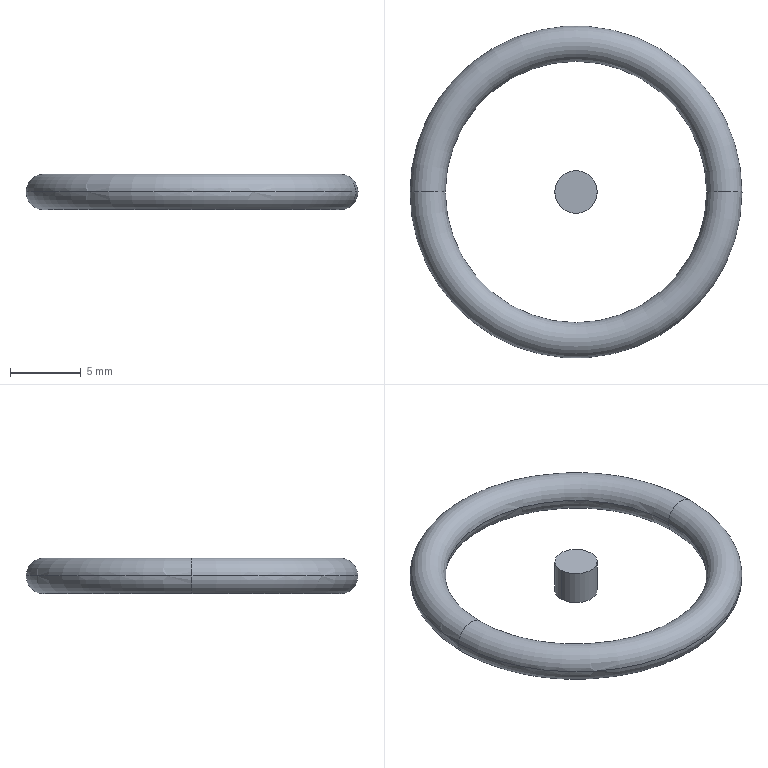Part | STEP file | O-ring 11 diameter after expansion 19 | 2 solids | 8 faces | box 23.5 x 23.5 x 2.5 mm | volume 341.518 mm3 | torus 4 | cylinder 2 | plane 2 | commonest cylinder face diameters 3 x2
STEP:
#1=CARTESIAN_POINT('',(0.,0.,0.));
#2=DIRECTION('',(0.,0.,1.));
#3=DIRECTION('',(1.,0.,0.));
#4=AXIS2_PLACEMENT_3D('',#1,#2,#3);
#5=CARTESIAN_POINT('',(-11.75,0.,0.));
#6=VERTEX_POINT('',#5);
#7=CARTESIAN_POINT('',(-9.25,0.,0.));
#8=VERTEX_POINT('',#7);
#9=CARTESIAN_POINT('',(-10.5,0.,0.));
#10=DIRECTION('',(0.,1.,0.));
#11=DIRECTION('',(-1.,0.,0.));
#12=AXIS2_PLACEMENT_3D('',#9,#10,#11);
#13=CIRCLE('',#12,1.25);
#14=CARTESIAN_POINT('',(0.,0.,0.));
#15=DIRECTION('',(0.,0.,1.));
#16=DIRECTION('',(1.,0.,0.));
#17=AXIS2_PLACEMENT_3D('',#14,#15,#16);
#18=TOROIDAL_SURFACE('',#17,10.5,1.25);
#19=CARTESIAN_POINT('',(3.142,0.));
#20=DIRECTION('',(0.,1.));
#21=VECTOR('',#20,1.);
#22=LINE('',#19,#21);
#23=(GEOMETRIC_REPRESENTATION_CONTEXT(2)PARAMETRIC_REPRESENTATION_CONTEXT()REPRESENTATION_CONTEXT('',''));
#24=DEFINITIONAL_REPRESENTATION('',(#22),#23);
#25=PCURVE('',#18,#24);
#26=CARTESIAN_POINT('',(0.,0.,0.));
#27=DIRECTION('',(0.,0.,1.));
#28=DIRECTION('',(1.,0.,0.));
#29=AXIS2_PLACEMENT_3D('',#26,#27,#28);
#30=TOROIDAL_SURFACE('',#29,10.5,1.25);
#31=CARTESIAN_POINT('',(3.142,0.));
#32=DIRECTION('',(0.,1.));
#33=VECTOR('',#32,1.);
#34=LINE('',#31,#33);
#35=(GEOMETRIC_REPRESENTATION_CONTEXT(2)PARAMETRIC_REPRESENTATION_CONTEXT()REPRESENTATION_CONTEXT('',''));
#36=DEFINITIONAL_REPRESENTATION('',(#34),#35);
#37=PCURVE('',#30,#36);
#38=SURFACE_CURVE('',#13,(#25,#37),.PCURVE_S1.);
#39=EDGE_CURVE('',#6,#8,#38,.T.);
#40=ORIENTED_EDGE('',*,*,#39,.F.);
#41=CARTESIAN_POINT('',(11.75,0.,0.));
#42=VERTEX_POINT('',#41);
#43=CARTESIAN_POINT('',(0.,0.,0.));
#44=DIRECTION('',(0.,0.,1.));
#45=DIRECTION('',(1.,0.,0.));
#46=AXIS2_PLACEMENT_3D('',#43,#44,#45);
#47=CIRCLE('',#46,11.75);
#48=CARTESIAN_POINT('',(0.,0.));
#49=DIRECTION('',(1.,0.));
#50=VECTOR('',#49,1.);
#51=LINE('',#48,#50);
#52=(GEOMETRIC_REPRESENTATION_CONTEXT(2)PARAMETRIC_REPRESENTATION_CONTEXT()REPRESENTATION_CONTEXT('',''));
#53=DEFINITIONAL_REPRESENTATION('',(#51),#52);
#54=PCURVE('',#18,#53);
#55=CARTESIAN_POINT('',(0.,0.,0.));
#56=DIRECTION('',(0.,0.,1.));
#57=DIRECTION('',(1.,0.,0.));
#58=AXIS2_PLACEMENT_3D('',#55,#56,#57);
#59=TOROIDAL_SURFACE('',#58,10.5,1.25);
#60=CARTESIAN_POINT('',(0.,6.283));
#61=DIRECTION('',(1.,0.));
#62=VECTOR('',#61,1.);
#63=LINE('',#60,#62);
#64=(GEOMETRIC_REPRESENTATION_CONTEXT(2)PARAMETRIC_REPRESENTATION_CONTEXT()REPRESENTATION_CONTEXT('',''));
#65=DEFINITIONAL_REPRESENTATION('',(#63),#64);
#66=PCURVE('',#59,#65);
#67=SURFACE_CURVE('',#47,(#54,#66),.PCURVE_S1.);
#68=EDGE_CURVE('',#6,#42,#67,.T.);
#69=ORIENTED_EDGE('',*,*,#68,.T.);
#70=CARTESIAN_POINT('',(9.25,0.,0.));
#71=VERTEX_POINT('',#70);
#72=CARTESIAN_POINT('',(10.5,0.,0.));
#73=DIRECTION('',(0.,-1.,0.));
#74=DIRECTION('',(0.,0.,-1.));
#75=AXIS2_PLACEMENT_3D('',#72,#73,#74);
#76=CIRCLE('',#75,1.25);
#77=CARTESIAN_POINT('',(6.283,-1.571));
#78=DIRECTION('',(0.,1.));
#79=VECTOR('',#78,1.);
#80=LINE('',#77,#79);
#81=(GEOMETRIC_REPRESENTATION_CONTEXT(2)PARAMETRIC_REPRESENTATION_CONTEXT()REPRESENTATION_CONTEXT('',''));
#82=DEFINITIONAL_REPRESENTATION('',(#80),#81);
#83=PCURVE('',#18,#82);
#84=CARTESIAN_POINT('',(0.,-1.571));
#85=DIRECTION('',(0.,1.));
#86=VECTOR('',#85,1.);
#87=LINE('',#84,#86);
#88=(GEOMETRIC_REPRESENTATION_CONTEXT(2)PARAMETRIC_REPRESENTATION_CONTEXT()REPRESENTATION_CONTEXT('',''));
#89=DEFINITIONAL_REPRESENTATION('',(#87),#88);
#90=PCURVE('',#30,#89);
#91=SURFACE_CURVE('',#76,(#83,#90),.PCURVE_S1.);
#92=EDGE_CURVE('',#42,#71,#91,.T.);
#93=ORIENTED_EDGE('',*,*,#92,.T.);
#94=CARTESIAN_POINT('',(0.,0.,0.));
#95=DIRECTION('',(0.,0.,1.));
#96=DIRECTION('',(1.,0.,0.));
#97=AXIS2_PLACEMENT_3D('',#94,#95,#96);
#98=CIRCLE('',#97,9.25);
#99=CARTESIAN_POINT('',(0.,3.142));
#100=DIRECTION('',(1.,0.));
#101=VECTOR('',#100,1.);
#102=LINE('',#99,#101);
#103=(GEOMETRIC_REPRESENTATION_CONTEXT(2)PARAMETRIC_REPRESENTATION_CONTEXT()REPRESENTATION_CONTEXT('',''));
#104=DEFINITIONAL_REPRESENTATION('',(#102),#103);
#105=PCURVE('',#18,#104);
#106=CARTESIAN_POINT('',(0.,3.142));
#107=DIRECTION('',(1.,0.));
#108=VECTOR('',#107,1.);
#109=LINE('',#106,#108);
#110=(GEOMETRIC_REPRESENTATION_CONTEXT(2)PARAMETRIC_REPRESENTATION_CONTEXT()REPRESENTATION_CONTEXT('',''));
#111=DEFINITIONAL_REPRESENTATION('',(#109),#110);
#112=PCURVE('',#59,#111);
#113=SURFACE_CURVE('',#98,(#105,#112),.PCURVE_S1.);
#114=EDGE_CURVE('',#8,#71,#113,.T.);
#115=ORIENTED_EDGE('',*,*,#114,.F.);
#116=EDGE_LOOP('',(#40,#69,#93,#115));
#117=FACE_BOUND('',#116,.T.);
#118=ADVANCED_FACE('',(#117),#18,.T.);
#119=ORIENTED_EDGE('',*,*,#92,.F.);
#120=CARTESIAN_POINT('',(0.,0.,0.));
#121=DIRECTION('',(0.,0.,1.));
#122=DIRECTION('',(1.,0.,0.));
#123=AXIS2_PLACEMENT_3D('',#120,#121,#122);
#124=CIRCLE('',#123,11.75);
#125=CARTESIAN_POINT('',(0.,0.));
#126=DIRECTION('',(1.,0.));
#127=VECTOR('',#126,1.);
#128=LINE('',#125,#127);
#129=(GEOMETRIC_REPRESENTATION_CONTEXT(2)PARAMETRIC_REPRESENTATION_CONTEXT()REPRESENTATION_CONTEXT('',''));
#130=DEFINITIONAL_REPRESENTATION('',(#128),#129);
#131=PCURVE('',#30,#130);
#132=CARTESIAN_POINT('',(0.,0.,0.));
#133=DIRECTION('',(0.,0.,1.));
#134=DIRECTION('',(1.,0.,0.));
#135=AXIS2_PLACEMENT_3D('',#132,#133,#134);
#136=TOROIDAL_SURFACE('',#135,10.5,1.25);
#137=CARTESIAN_POINT('',(0.,6.283));
#138=DIRECTION('',(1.,0.));
#139=VECTOR('',#138,1.);
#140=LINE('',#137,#139);
#141=(GEOMETRIC_REPRESENTATION_CONTEXT(2)PARAMETRIC_REPRESENTATION_CONTEXT()REPRESENTATION_CONTEXT('',''));
#142=DEFINITIONAL_REPRESENTATION('',(#140),#141);
#143=PCURVE('',#136,#142);
#144=SURFACE_CURVE('',#124,(#131,#143),.PCURVE_S1.);
#145=EDGE_CURVE('',#42,#6,#144,.T.);
#146=ORIENTED_EDGE('',*,*,#145,.T.);
#147=ORIENTED_EDGE('',*,*,#39,.T.);
#148=CARTESIAN_POINT('',(0.,0.,0.));
#149=DIRECTION('',(0.,0.,1.));
#150=DIRECTION('',(1.,0.,0.));
#151=AXIS2_PLACEMENT_3D('',#148,#149,#150);
#152=CIRCLE('',#151,9.25);
#153=CARTESIAN_POINT('',(0.,3.142));
#154=DIRECTION('',(1.,0.));
#155=VECTOR('',#154,1.);
#156=LINE('',#153,#155);
#157=(GEOMETRIC_REPRESENTATION_CONTEXT(2)PARAMETRIC_REPRESENTATION_CONTEXT()REPRESENTATION_CONTEXT('',''));
#158=DEFINITIONAL_REPRESENTATION('',(#156),#157);
#159=PCURVE('',#30,#158);
#160=CARTESIAN_POINT('',(0.,3.142));
#161=DIRECTION('',(1.,0.));
#162=VECTOR('',#161,1.);
#163=LINE('',#160,#162);
#164=(GEOMETRIC_REPRESENTATION_CONTEXT(2)PARAMETRIC_REPRESENTATION_CONTEXT()REPRESENTATION_CONTEXT('',''));
#165=DEFINITIONAL_REPRESENTATION('',(#163),#164);
#166=PCURVE('',#136,#165);
#167=SURFACE_CURVE('',#152,(#159,#166),.PCURVE_S1.);
#168=EDGE_CURVE('',#71,#8,#167,.T.);
#169=ORIENTED_EDGE('',*,*,#168,.F.);
#170=EDGE_LOOP('',(#119,#146,#147,#169));
#171=FACE_BOUND('',#170,.T.);
#172=ADVANCED_FACE('',(#171),#30,.T.);
#173=ORIENTED_EDGE('',*,*,#145,.F.);
#174=CARTESIAN_POINT('',(10.5,0.,0.));
#175=DIRECTION('',(0.,-1.,0.));
#176=DIRECTION('',(0.,0.,-1.));
#177=AXIS2_PLACEMENT_3D('',#174,#175,#176);
#178=CIRCLE('',#177,1.25);
#179=CARTESIAN_POINT('',(0.,-1.571));
#180=DIRECTION('',(0.,1.));
#181=VECTOR('',#180,1.);
#182=LINE('',#179,#181);
#183=(GEOMETRIC_REPRESENTATION_CONTEXT(2)PARAMETRIC_REPRESENTATION_CONTEXT()REPRESENTATION_CONTEXT('',''));
#184=DEFINITIONAL_REPRESENTATION('',(#182),#183);
#185=PCURVE('',#136,#184);
#186=CARTESIAN_POINT('',(6.283,-1.571));
#187=DIRECTION('',(0.,1.));
#188=VECTOR('',#187,1.);
#189=LINE('',#186,#188);
#190=(GEOMETRIC_REPRESENTATION_CONTEXT(2)PARAMETRIC_REPRESENTATION_CONTEXT()REPRESENTATION_CONTEXT('',''));
#191=DEFINITIONAL_REPRESENTATION('',(#189),#190);
#192=PCURVE('',#59,#191);
#193=SURFACE_CURVE('',#178,(#185,#192),.PCURVE_S1.);
#194=EDGE_CURVE('',#71,#42,#193,.T.);
#195=ORIENTED_EDGE('',*,*,#194,.F.);
#196=ORIENTED_EDGE('',*,*,#168,.T.);
#197=CARTESIAN_POINT('',(-10.5,0.,0.));
#198=DIRECTION('',(0.,1.,0.));
#199=DIRECTION('',(-1.,0.,0.));
#200=AXIS2_PLACEMENT_3D('',#197,#198,#199);
#201=CIRCLE('',#200,1.25);
#202=CARTESIAN_POINT('',(3.142,0.));
#203=DIRECTION('',(0.,1.));
#204=VECTOR('',#203,1.);
#205=LINE('',#202,#204);
#206=(GEOMETRIC_REPRESENTATION_CONTEXT(2)PARAMETRIC_REPRESENTATION_CONTEXT()REPRESENTATION_CONTEXT('',''));
#207=DEFINITIONAL_REPRESENTATION('',(#205),#206);
#208=PCURVE('',#136,#207);
#209=CARTESIAN_POINT('',(3.142,0.));
#210=DIRECTION('',(0.,1.));
#211=VECTOR('',#210,1.);
#212=LINE('',#209,#211);
#213=(GEOMETRIC_REPRESENTATION_CONTEXT(2)PARAMETRIC_REPRESENTATION_CONTEXT()REPRESENTATION_CONTEXT('',''));
#214=DEFINITIONAL_REPRESENTATION('',(#212),#213);
#215=PCURVE('',#59,#214);
#216=SURFACE_CURVE('',#201,(#208,#215),.PCURVE_S1.);
#217=EDGE_CURVE('',#8,#6,#216,.T.);
#218=ORIENTED_EDGE('',*,*,#217,.T.);
#219=EDGE_LOOP('',(#173,#195,#196,#218));
#220=FACE_BOUND('',#219,.T.);
#221=ADVANCED_FACE('',(#220),#136,.T.);
#222=ORIENTED_EDGE('',*,*,#68,.F.);
#223=ORIENTED_EDGE('',*,*,#217,.F.);
#224=ORIENTED_EDGE('',*,*,#114,.T.);
#225=ORIENTED_EDGE('',*,*,#194,.T.);
#226=EDGE_LOOP('',(#222,#223,#224,#225));
#227=FACE_BOUND('',#226,.T.);
#228=ADVANCED_FACE('',(#227),#59,.T.);
#229=CLOSED_SHELL('',(#118,#172,#221,#228));
#230=MANIFOLD_SOLID_BREP('',#229);
#231=CARTESIAN_POINT('',(1.5,0.,-1.25));
#232=VERTEX_POINT('',#231);
#233=CARTESIAN_POINT('',(-1.5,0.,-1.25));
#234=VERTEX_POINT('',#233);
#235=CARTESIAN_POINT('',(0.,0.,-1.25));
#236=DIRECTION('',(0.,0.,1.));
#237=DIRECTION('',(1.,0.,0.));
#238=AXIS2_PLACEMENT_3D('',#235,#236,#237);
#239=CIRCLE('',#238,1.5);
#240=CARTESIAN_POINT('',(0.,0.,-1.25));
#241=DIRECTION('',(0.,0.,1.));
#242=DIRECTION('',(1.,0.,0.));
#243=AXIS2_PLACEMENT_3D('',#240,#241,#242);
#244=CYLINDRICAL_SURFACE('',#243,1.5);
#245=CARTESIAN_POINT('',(0.,0.));
#246=DIRECTION('',(1.,0.));
#247=VECTOR('',#246,1.);
#248=LINE('',#245,#247);
#249=(GEOMETRIC_REPRESENTATION_CONTEXT(2)PARAMETRIC_REPRESENTATION_CONTEXT()REPRESENTATION_CONTEXT('',''));
#250=DEFINITIONAL_REPRESENTATION('',(#248),#249);
#251=PCURVE('',#244,#250);
#252=CARTESIAN_POINT('',(0.,0.,-1.25));
#253=DIRECTION('',(0.,0.,1.));
#254=DIRECTION('',(1.,0.,0.));
#255=AXIS2_PLACEMENT_3D('',#252,#253,#254);
#256=PLANE('',#255);
#257=CARTESIAN_POINT('',(0.,0.));
#258=DIRECTION('',(1.,0.));
#259=AXIS2_PLACEMENT_2D('',#257,#258);
#260=CIRCLE('',#259,1.5);
#261=(GEOMETRIC_REPRESENTATION_CONTEXT(2)PARAMETRIC_REPRESENTATION_CONTEXT()REPRESENTATION_CONTEXT('',''));
#262=DEFINITIONAL_REPRESENTATION('',(#260),#261);
#263=PCURVE('',#256,#262);
#264=SURFACE_CURVE('',#239,(#251,#263),.PCURVE_S1.);
#265=EDGE_CURVE('',#232,#234,#264,.T.);
#266=ORIENTED_EDGE('',*,*,#265,.T.);
#267=CARTESIAN_POINT('',(-1.5,0.,1.25));
#268=VERTEX_POINT('',#267);
#269=CARTESIAN_POINT('',(-1.5,0.,-1.25));
#270=DIRECTION('',(0.,0.,1.));
#271=VECTOR('',#270,1.);
#272=LINE('',#269,#271);
#273=CARTESIAN_POINT('',(3.142,0.));
#274=DIRECTION('',(0.,1.));
#275=VECTOR('',#274,1.);
#276=LINE('',#273,#275);
#277=(GEOMETRIC_REPRESENTATION_CONTEXT(2)PARAMETRIC_REPRESENTATION_CONTEXT()REPRESENTATION_CONTEXT('',''));
#278=DEFINITIONAL_REPRESENTATION('',(#276),#277);
#279=PCURVE('',#244,#278);
#280=CARTESIAN_POINT('',(0.,0.,-1.25));
#281=DIRECTION('',(0.,0.,1.));
#282=DIRECTION('',(1.,0.,0.));
#283=AXIS2_PLACEMENT_3D('',#280,#281,#282);
#284=CYLINDRICAL_SURFACE('',#283,1.5);
#285=CARTESIAN_POINT('',(3.142,0.));
#286=DIRECTION('',(0.,1.));
#287=VECTOR('',#286,1.);
#288=LINE('',#285,#287);
#289=(GEOMETRIC_REPRESENTATION_CONTEXT(2)PARAMETRIC_REPRESENTATION_CONTEXT()REPRESENTATION_CONTEXT('',''));
#290=DEFINITIONAL_REPRESENTATION('',(#288),#289);
#291=PCURVE('',#284,#290);
#292=SURFACE_CURVE('',#272,(#279,#291),.PCURVE_S1.);
#293=EDGE_CURVE('',#234,#268,#292,.T.);
#294=ORIENTED_EDGE('',*,*,#293,.T.);
#295=CARTESIAN_POINT('',(1.5,0.,1.25));
#296=VERTEX_POINT('',#295);
#297=CARTESIAN_POINT('',(0.,0.,1.25));
#298=DIRECTION('',(0.,0.,1.));
#299=DIRECTION('',(1.,0.,0.));
#300=AXIS2_PLACEMENT_3D('',#297,#298,#299);
#301=CIRCLE('',#300,1.5);
#302=CARTESIAN_POINT('',(0.,2.5));
#303=DIRECTION('',(1.,0.));
#304=VECTOR('',#303,1.);
#305=LINE('',#302,#304);
#306=(GEOMETRIC_REPRESENTATION_CONTEXT(2)PARAMETRIC_REPRESENTATION_CONTEXT()REPRESENTATION_CONTEXT('',''));
#307=DEFINITIONAL_REPRESENTATION('',(#305),#306);
#308=PCURVE('',#244,#307);
#309=CARTESIAN_POINT('',(0.,0.,1.25));
#310=DIRECTION('',(0.,0.,1.));
#311=DIRECTION('',(1.,0.,0.));
#312=AXIS2_PLACEMENT_3D('',#309,#310,#311);
#313=PLANE('',#312);
#314=CARTESIAN_POINT('',(0.,0.));
#315=DIRECTION('',(1.,0.));
#316=AXIS2_PLACEMENT_2D('',#314,#315);
#317=CIRCLE('',#316,1.5);
#318=(GEOMETRIC_REPRESENTATION_CONTEXT(2)PARAMETRIC_REPRESENTATION_CONTEXT()REPRESENTATION_CONTEXT('',''));
#319=DEFINITIONAL_REPRESENTATION('',(#317),#318);
#320=PCURVE('',#313,#319);
#321=SURFACE_CURVE('',#301,(#308,#320),.PCURVE_S1.);
#322=EDGE_CURVE('',#296,#268,#321,.T.);
#323=ORIENTED_EDGE('',*,*,#322,.F.);
#324=CARTESIAN_POINT('',(1.5,0.,-1.25));
#325=DIRECTION('',(0.,0.,1.));
#326=VECTOR('',#325,1.);
#327=LINE('',#324,#326);
#328=CARTESIAN_POINT('',(0.,0.));
#329=DIRECTION('',(0.,1.));
#330=VECTOR('',#329,1.);
#331=LINE('',#328,#330);
#332=(GEOMETRIC_REPRESENTATION_CONTEXT(2)PARAMETRIC_REPRESENTATION_CONTEXT()REPRESENTATION_CONTEXT('',''));
#333=DEFINITIONAL_REPRESENTATION('',(#331),#332);
#334=PCURVE('',#244,#333);
#335=CARTESIAN_POINT('',(6.283,0.));
#336=DIRECTION('',(0.,1.));
#337=VECTOR('',#336,1.);
#338=LINE('',#335,#337);
#339=(GEOMETRIC_REPRESENTATION_CONTEXT(2)PARAMETRIC_REPRESENTATION_CONTEXT()REPRESENTATION_CONTEXT('',''));
#340=DEFINITIONAL_REPRESENTATION('',(#338),#339);
#341=PCURVE('',#284,#340);
#342=SURFACE_CURVE('',#327,(#334,#341),.PCURVE_S1.);
#343=EDGE_CURVE('',#232,#296,#342,.T.);
#344=ORIENTED_EDGE('',*,*,#343,.F.);
#345=EDGE_LOOP('',(#266,#294,#323,#344));
#346=FACE_BOUND('',#345,.T.);
#347=ADVANCED_FACE('',(#346),#244,.T.);
#348=ORIENTED_EDGE('',*,*,#293,.F.);
#349=CARTESIAN_POINT('',(0.,0.,-1.25));
#350=DIRECTION('',(0.,0.,1.));
#351=DIRECTION('',(1.,0.,0.));
#352=AXIS2_PLACEMENT_3D('',#349,#350,#351);
#353=CIRCLE('',#352,1.5);
#354=CARTESIAN_POINT('',(0.,0.));
#355=DIRECTION('',(1.,0.));
#356=VECTOR('',#355,1.);
#357=LINE('',#354,#356);
#358=(GEOMETRIC_REPRESENTATION_CONTEXT(2)PARAMETRIC_REPRESENTATION_CONTEXT()REPRESENTATION_CONTEXT('',''));
#359=DEFINITIONAL_REPRESENTATION('',(#357),#358);
#360=PCURVE('',#284,#359);
#361=CARTESIAN_POINT('',(0.,0.));
#362=DIRECTION('',(1.,0.));
#363=AXIS2_PLACEMENT_2D('',#361,#362);
#364=CIRCLE('',#363,1.5);
#365=(GEOMETRIC_REPRESENTATION_CONTEXT(2)PARAMETRIC_REPRESENTATION_CONTEXT()REPRESENTATION_CONTEXT('',''));
#366=DEFINITIONAL_REPRESENTATION('',(#364),#365);
#367=PCURVE('',#256,#366);
#368=SURFACE_CURVE('',#353,(#360,#367),.PCURVE_S1.);
#369=EDGE_CURVE('',#234,#232,#368,.T.);
#370=ORIENTED_EDGE('',*,*,#369,.T.);
#371=ORIENTED_EDGE('',*,*,#343,.T.);
#372=CARTESIAN_POINT('',(0.,0.,1.25));
#373=DIRECTION('',(0.,0.,1.));
#374=DIRECTION('',(1.,0.,0.));
#375=AXIS2_PLACEMENT_3D('',#372,#373,#374);
#376=CIRCLE('',#375,1.5);
#377=CARTESIAN_POINT('',(0.,2.5));
#378=DIRECTION('',(1.,0.));
#379=VECTOR('',#378,1.);
#380=LINE('',#377,#379);
#381=(GEOMETRIC_REPRESENTATION_CONTEXT(2)PARAMETRIC_REPRESENTATION_CONTEXT()REPRESENTATION_CONTEXT('',''));
#382=DEFINITIONAL_REPRESENTATION('',(#380),#381);
#383=PCURVE('',#284,#382);
#384=CARTESIAN_POINT('',(0.,0.));
#385=DIRECTION('',(1.,0.));
#386=AXIS2_PLACEMENT_2D('',#384,#385);
#387=CIRCLE('',#386,1.5);
#388=(GEOMETRIC_REPRESENTATION_CONTEXT(2)PARAMETRIC_REPRESENTATION_CONTEXT()REPRESENTATION_CONTEXT('',''));
#389=DEFINITIONAL_REPRESENTATION('',(#387),#388);
#390=PCURVE('',#313,#389);
#391=SURFACE_CURVE('',#376,(#383,#390),.PCURVE_S1.);
#392=EDGE_CURVE('',#268,#296,#391,.T.);
#393=ORIENTED_EDGE('',*,*,#392,.F.);
#394=EDGE_LOOP('',(#348,#370,#371,#393));
#395=FACE_BOUND('',#394,.T.);
#396=ADVANCED_FACE('',(#395),#284,.T.);
#397=ORIENTED_EDGE('',*,*,#265,.F.);
#398=ORIENTED_EDGE('',*,*,#369,.F.);
#399=EDGE_LOOP('',(#397,#398));
#400=FACE_BOUND('',#399,.T.);
#401=ADVANCED_FACE('',(#400),#256,.F.);
#402=ORIENTED_EDGE('',*,*,#322,.T.);
#403=ORIENTED_EDGE('',*,*,#392,.T.);
#404=EDGE_LOOP('',(#402,#403));
#405=FACE_BOUND('',#404,.T.);
#406=ADVANCED_FACE('',(#405),#313,.T.);
#407=CLOSED_SHELL('',(#347,#396,#401,#406));
#408=MANIFOLD_SOLID_BREP('',#407);
#409=(LENGTH_UNIT()NAMED_UNIT(*)SI_UNIT(.MILLI.,.METRE.));
#410=UNCERTAINTY_MEASURE_WITH_UNIT(LENGTH_MEASURE(0.0000001),#409,'','');
#411=(NAMED_UNIT(*)PLANE_ANGLE_UNIT()SI_UNIT($,.RADIAN.));
#412=(NAMED_UNIT(*)SI_UNIT($,.STERADIAN.)SOLID_ANGLE_UNIT());
#413=(GEOMETRIC_REPRESENTATION_CONTEXT(3)GLOBAL_UNCERTAINTY_ASSIGNED_CONTEXT((#410))GLOBAL_UNIT_ASSIGNED_CONTEXT((#409,#411,#412))REPRESENTATION_CONTEXT('',''));
#414=SHAPE_REPRESENTATION('',(#4,#230,#408),#413);